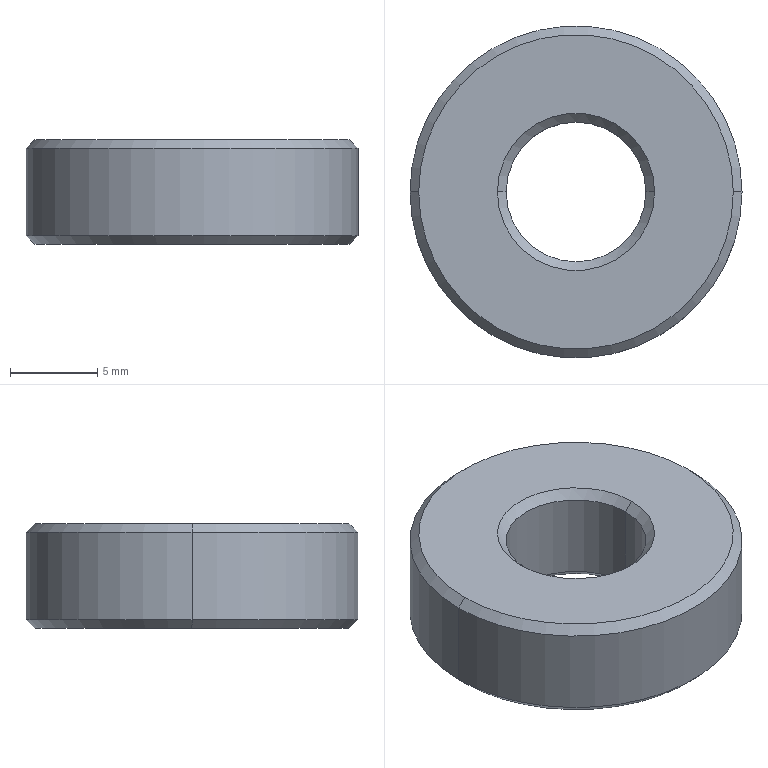Part | STEP file | QA-B698ZZ | 1 solid | 14 faces | box 19 x 19 x 6 mm | volume 1378 mm3 | cone 8 | cylinder 4 | plane 2 | commonest cylinder face diameters 8 x2 19 x2
STEP:
#1=CARTESIAN_POINT('',(0.,0.,0.));
#2=DIRECTION('',(0.,0.,1.));
#3=DIRECTION('',(1.,0.,0.));
#4=AXIS2_PLACEMENT_3D('',#1,#2,#3);
#5=CARTESIAN_POINT('',(4.,0.,5.5));
#6=VERTEX_POINT('',#5);
#7=CARTESIAN_POINT('',(4.5,0.,6.));
#8=VERTEX_POINT('',#7);
#9=CARTESIAN_POINT('',(4.,0.,5.5));
#10=DIRECTION('',(0.7071,0.,0.7071));
#11=VECTOR('',#10,1.);
#12=LINE('',#9,#11);
#13=CARTESIAN_POINT('',(0.,0.,5.5));
#14=DIRECTION('',(0.,0.,1.));
#15=DIRECTION('',(1.,0.,0.));
#16=AXIS2_PLACEMENT_3D('',#13,#14,#15);
#17=CONICAL_SURFACE('',#16,4.,0.7854);
#18=CARTESIAN_POINT('',(6.283,0.));
#19=DIRECTION('',(0.,1.));
#20=VECTOR('',#19,1.);
#21=LINE('',#18,#20);
#22=(GEOMETRIC_REPRESENTATION_CONTEXT(2)PARAMETRIC_REPRESENTATION_CONTEXT()REPRESENTATION_CONTEXT('',''));
#23=DEFINITIONAL_REPRESENTATION('',(#21),#22);
#24=PCURVE('',#17,#23);
#25=CARTESIAN_POINT('',(0.,0.,5.5));
#26=DIRECTION('',(0.,0.,1.));
#27=DIRECTION('',(1.,0.,0.));
#28=AXIS2_PLACEMENT_3D('',#25,#26,#27);
#29=CONICAL_SURFACE('',#28,4.,0.7854);
#30=CARTESIAN_POINT('',(0.,0.));
#31=DIRECTION('',(0.,1.));
#32=VECTOR('',#31,1.);
#33=LINE('',#30,#32);
#34=(GEOMETRIC_REPRESENTATION_CONTEXT(2)PARAMETRIC_REPRESENTATION_CONTEXT()REPRESENTATION_CONTEXT('',''));
#35=DEFINITIONAL_REPRESENTATION('',(#33),#34);
#36=PCURVE('',#29,#35);
#37=SURFACE_CURVE('',#12,(#24,#36),.PCURVE_S1.);
#38=EDGE_CURVE('',#6,#8,#37,.T.);
#39=ORIENTED_EDGE('',*,*,#38,.T.);
#40=CARTESIAN_POINT('',(-4.5,0.,6.));
#41=VERTEX_POINT('',#40);
#42=CARTESIAN_POINT('',(0.,0.,6.));
#43=DIRECTION('',(0.,0.,-1.));
#44=DIRECTION('',(1.,0.,0.));
#45=AXIS2_PLACEMENT_3D('',#42,#43,#44);
#46=CIRCLE('',#45,4.5);
#47=CARTESIAN_POINT('',(6.283,0.5));
#48=DIRECTION('',(-1.,0.));
#49=VECTOR('',#48,1.);
#50=LINE('',#47,#49);
#51=(GEOMETRIC_REPRESENTATION_CONTEXT(2)PARAMETRIC_REPRESENTATION_CONTEXT()REPRESENTATION_CONTEXT('',''));
#52=DEFINITIONAL_REPRESENTATION('',(#50),#51);
#53=PCURVE('',#17,#52);
#54=CARTESIAN_POINT('',(0.,0.,6.));
#55=DIRECTION('',(0.,0.,1.));
#56=DIRECTION('',(1.,0.,0.));
#57=AXIS2_PLACEMENT_3D('',#54,#55,#56);
#58=PLANE('',#57);
#59=CARTESIAN_POINT('',(4.5,0.));
#60=CARTESIAN_POINT('',(4.5,-7.794));
#61=CARTESIAN_POINT('',(-2.25,-3.897));
#62=CARTESIAN_POINT('',(-9.,0.));
#63=CARTESIAN_POINT('',(-2.25,3.897));
#64=CARTESIAN_POINT('',(4.5,7.794));
#65=CARTESIAN_POINT('',(4.5,0.));
#66=(BOUNDED_CURVE()B_SPLINE_CURVE(2,(#59,#60,#61,#62,#63,#64,#65),.UNSPECIFIED.,.T.,.F.)B_SPLINE_CURVE_WITH_KNOTS((1,2,2,2,2,1),(-2.094,0.,2.094,4.189,6.283,8.378),.UNSPECIFIED.)CURVE()GEOMETRIC_REPRESENTATION_ITEM()RATIONAL_B_SPLINE_CURVE((1.,0.5,1.,0.5,1.,0.5,1.))REPRESENTATION_ITEM(''));
#67=(GEOMETRIC_REPRESENTATION_CONTEXT(2)PARAMETRIC_REPRESENTATION_CONTEXT()REPRESENTATION_CONTEXT('',''));
#68=DEFINITIONAL_REPRESENTATION('',(#66),#67);
#69=PCURVE('',#58,#68);
#70=SURFACE_CURVE('',#46,(#53,#69),.PCURVE_S1.);
#71=EDGE_CURVE('',#8,#41,#70,.T.);
#72=ORIENTED_EDGE('',*,*,#71,.T.);
#73=CARTESIAN_POINT('',(-4.,0.,5.5));
#74=VERTEX_POINT('',#73);
#75=CARTESIAN_POINT('',(-4.,0.,5.5));
#76=DIRECTION('',(-0.7071,0.,0.7071));
#77=VECTOR('',#76,1.);
#78=LINE('',#75,#77);
#79=CARTESIAN_POINT('',(3.142,0.));
#80=DIRECTION('',(0.,1.));
#81=VECTOR('',#80,1.);
#82=LINE('',#79,#81);
#83=(GEOMETRIC_REPRESENTATION_CONTEXT(2)PARAMETRIC_REPRESENTATION_CONTEXT()REPRESENTATION_CONTEXT('',''));
#84=DEFINITIONAL_REPRESENTATION('',(#82),#83);
#85=PCURVE('',#17,#84);
#86=CARTESIAN_POINT('',(3.142,0.));
#87=DIRECTION('',(0.,1.));
#88=VECTOR('',#87,1.);
#89=LINE('',#86,#88);
#90=(GEOMETRIC_REPRESENTATION_CONTEXT(2)PARAMETRIC_REPRESENTATION_CONTEXT()REPRESENTATION_CONTEXT('',''));
#91=DEFINITIONAL_REPRESENTATION('',(#89),#90);
#92=PCURVE('',#29,#91);
#93=SURFACE_CURVE('',#78,(#85,#92),.PCURVE_S1.);
#94=EDGE_CURVE('',#74,#41,#93,.T.);
#95=ORIENTED_EDGE('',*,*,#94,.F.);
#96=CARTESIAN_POINT('',(0.,0.,5.5));
#97=DIRECTION('',(0.,0.,1.));
#98=DIRECTION('',(1.,0.,0.));
#99=AXIS2_PLACEMENT_3D('',#96,#97,#98);
#100=CIRCLE('',#99,4.);
#101=CARTESIAN_POINT('',(0.,0.));
#102=DIRECTION('',(1.,0.));
#103=VECTOR('',#102,1.);
#104=LINE('',#101,#103);
#105=(GEOMETRIC_REPRESENTATION_CONTEXT(2)PARAMETRIC_REPRESENTATION_CONTEXT()REPRESENTATION_CONTEXT('',''));
#106=DEFINITIONAL_REPRESENTATION('',(#104),#105);
#107=PCURVE('',#17,#106);
#108=CARTESIAN_POINT('',(0.,0.,6.));
#109=DIRECTION('',(0.,0.,-1.));
#110=DIRECTION('',(-1.,0.,0.));
#111=AXIS2_PLACEMENT_3D('',#108,#109,#110);
#112=CYLINDRICAL_SURFACE('',#111,4.);
#113=CARTESIAN_POINT('',(9.425,0.5));
#114=DIRECTION('',(-1.,0.));
#115=VECTOR('',#114,1.);
#116=LINE('',#113,#115);
#117=(GEOMETRIC_REPRESENTATION_CONTEXT(2)PARAMETRIC_REPRESENTATION_CONTEXT()REPRESENTATION_CONTEXT('',''));
#118=DEFINITIONAL_REPRESENTATION('',(#116),#117);
#119=PCURVE('',#112,#118);
#120=SURFACE_CURVE('',#100,(#107,#119),.PCURVE_S1.);
#121=EDGE_CURVE('',#74,#6,#120,.T.);
#122=ORIENTED_EDGE('',*,*,#121,.T.);
#123=EDGE_LOOP('',(#39,#72,#95,#122));
#124=FACE_BOUND('',#123,.F.);
#125=ADVANCED_FACE('',(#124),#17,.F.);
#126=CARTESIAN_POINT('',(-4.,0.,0.5));
#127=VERTEX_POINT('',#126);
#128=CARTESIAN_POINT('',(-4.5,0.,0.));
#129=VERTEX_POINT('',#128);
#130=CARTESIAN_POINT('',(-4.5,0.,0.));
#131=DIRECTION('',(-0.7071,0.,-0.7071));
#132=VECTOR('',#131,1.);
#133=LINE('',#130,#132);
#134=CARTESIAN_POINT('',(0.,0.,0.));
#135=DIRECTION('',(0.,0.,-1.));
#136=DIRECTION('',(-1.,0.,0.));
#137=AXIS2_PLACEMENT_3D('',#134,#135,#136);
#138=CONICAL_SURFACE('',#137,4.5,0.7854);
#139=CARTESIAN_POINT('',(6.283,0.));
#140=DIRECTION('',(0.,1.));
#141=VECTOR('',#140,1.);
#142=LINE('',#139,#141);
#143=(GEOMETRIC_REPRESENTATION_CONTEXT(2)PARAMETRIC_REPRESENTATION_CONTEXT()REPRESENTATION_CONTEXT('',''));
#144=DEFINITIONAL_REPRESENTATION('',(#142),#143);
#145=PCURVE('',#138,#144);
#146=CARTESIAN_POINT('',(0.,0.,0.));
#147=DIRECTION('',(0.,0.,-1.));
#148=DIRECTION('',(-1.,0.,0.));
#149=AXIS2_PLACEMENT_3D('',#146,#147,#148);
#150=CONICAL_SURFACE('',#149,4.5,0.7854);
#151=CARTESIAN_POINT('',(0.,0.));
#152=DIRECTION('',(0.,1.));
#153=VECTOR('',#152,1.);
#154=LINE('',#151,#153);
#155=(GEOMETRIC_REPRESENTATION_CONTEXT(2)PARAMETRIC_REPRESENTATION_CONTEXT()REPRESENTATION_CONTEXT('',''));
#156=DEFINITIONAL_REPRESENTATION('',(#154),#155);
#157=PCURVE('',#150,#156);
#158=SURFACE_CURVE('',#133,(#145,#157),.PCURVE_S1.);
#159=EDGE_CURVE('',#127,#129,#158,.T.);
#160=ORIENTED_EDGE('',*,*,#159,.T.);
#161=CARTESIAN_POINT('',(4.5,0.,0.));
#162=VERTEX_POINT('',#161);
#163=CARTESIAN_POINT('',(0.,0.,0.));
#164=DIRECTION('',(0.,0.,1.));
#165=DIRECTION('',(1.,0.,0.));
#166=AXIS2_PLACEMENT_3D('',#163,#164,#165);
#167=CIRCLE('',#166,4.5);
#168=CARTESIAN_POINT('',(9.425,0.));
#169=DIRECTION('',(-1.,0.));
#170=VECTOR('',#169,1.);
#171=LINE('',#168,#170);
#172=(GEOMETRIC_REPRESENTATION_CONTEXT(2)PARAMETRIC_REPRESENTATION_CONTEXT()REPRESENTATION_CONTEXT('',''));
#173=DEFINITIONAL_REPRESENTATION('',(#171),#172);
#174=PCURVE('',#138,#173);
#175=CARTESIAN_POINT('',(0.,0.,0.));
#176=DIRECTION('',(0.,0.,1.));
#177=DIRECTION('',(1.,0.,0.));
#178=AXIS2_PLACEMENT_3D('',#175,#176,#177);
#179=PLANE('',#178);
#180=CARTESIAN_POINT('',(0.,0.));
#181=DIRECTION('',(1.,0.));
#182=AXIS2_PLACEMENT_2D('',#180,#181);
#183=CIRCLE('',#182,4.5);
#184=(GEOMETRIC_REPRESENTATION_CONTEXT(2)PARAMETRIC_REPRESENTATION_CONTEXT()REPRESENTATION_CONTEXT('',''));
#185=DEFINITIONAL_REPRESENTATION('',(#183),#184);
#186=PCURVE('',#179,#185);
#187=SURFACE_CURVE('',#167,(#174,#186),.PCURVE_S1.);
#188=EDGE_CURVE('',#129,#162,#187,.T.);
#189=ORIENTED_EDGE('',*,*,#188,.T.);
#190=CARTESIAN_POINT('',(4.,0.,0.5));
#191=VERTEX_POINT('',#190);
#192=CARTESIAN_POINT('',(4.5,0.,0.));
#193=DIRECTION('',(0.7071,0.,-0.7071));
#194=VECTOR('',#193,1.);
#195=LINE('',#192,#194);
#196=CARTESIAN_POINT('',(3.142,0.));
#197=DIRECTION('',(0.,1.));
#198=VECTOR('',#197,1.);
#199=LINE('',#196,#198);
#200=(GEOMETRIC_REPRESENTATION_CONTEXT(2)PARAMETRIC_REPRESENTATION_CONTEXT()REPRESENTATION_CONTEXT('',''));
#201=DEFINITIONAL_REPRESENTATION('',(#199),#200);
#202=PCURVE('',#138,#201);
#203=CARTESIAN_POINT('',(3.142,0.));
#204=DIRECTION('',(0.,1.));
#205=VECTOR('',#204,1.);
#206=LINE('',#203,#205);
#207=(GEOMETRIC_REPRESENTATION_CONTEXT(2)PARAMETRIC_REPRESENTATION_CONTEXT()REPRESENTATION_CONTEXT('',''));
#208=DEFINITIONAL_REPRESENTATION('',(#206),#207);
#209=PCURVE('',#150,#208);
#210=SURFACE_CURVE('',#195,(#202,#209),.PCURVE_S1.);
#211=EDGE_CURVE('',#191,#162,#210,.T.);
#212=ORIENTED_EDGE('',*,*,#211,.F.);
#213=CARTESIAN_POINT('',(0.,0.,0.5));
#214=DIRECTION('',(0.,0.,-1.));
#215=DIRECTION('',(1.,0.,0.));
#216=AXIS2_PLACEMENT_3D('',#213,#214,#215);
#217=CIRCLE('',#216,4.);
#218=CARTESIAN_POINT('',(3.142,-0.5));
#219=DIRECTION('',(1.,0.));
#220=VECTOR('',#219,1.);
#221=LINE('',#218,#220);
#222=(GEOMETRIC_REPRESENTATION_CONTEXT(2)PARAMETRIC_REPRESENTATION_CONTEXT()REPRESENTATION_CONTEXT('',''));
#223=DEFINITIONAL_REPRESENTATION('',(#221),#222);
#224=PCURVE('',#138,#223);
#225=CARTESIAN_POINT('',(3.142,5.5));
#226=DIRECTION('',(1.,0.));
#227=VECTOR('',#226,1.);
#228=LINE('',#225,#227);
#229=(GEOMETRIC_REPRESENTATION_CONTEXT(2)PARAMETRIC_REPRESENTATION_CONTEXT()REPRESENTATION_CONTEXT('',''));
#230=DEFINITIONAL_REPRESENTATION('',(#228),#229);
#231=PCURVE('',#112,#230);
#232=SURFACE_CURVE('',#217,(#224,#231),.PCURVE_S1.);
#233=EDGE_CURVE('',#191,#127,#232,.T.);
#234=ORIENTED_EDGE('',*,*,#233,.T.);
#235=EDGE_LOOP('',(#160,#189,#212,#234));
#236=FACE_BOUND('',#235,.F.);
#237=ADVANCED_FACE('',(#236),#138,.F.);
#238=CARTESIAN_POINT('',(9.,0.,6.));
#239=VERTEX_POINT('',#238);
#240=CARTESIAN_POINT('',(-9.,0.,6.));
#241=VERTEX_POINT('',#240);
#242=CARTESIAN_POINT('',(0.,0.,6.));
#243=DIRECTION('',(0.,0.,1.));
#244=DIRECTION('',(1.,0.,0.));
#245=AXIS2_PLACEMENT_3D('',#242,#243,#244);
#246=CIRCLE('',#245,9.);
#247=CARTESIAN_POINT('',(0.,0.,6.));
#248=DIRECTION('',(0.,0.,-1.));
#249=DIRECTION('',(-1.,0.,0.));
#250=AXIS2_PLACEMENT_3D('',#247,#248,#249);
#251=CONICAL_SURFACE('',#250,9.,0.7854);
#252=CARTESIAN_POINT('',(3.142,0.));
#253=DIRECTION('',(-1.,0.));
#254=VECTOR('',#253,1.);
#255=LINE('',#252,#254);
#256=(GEOMETRIC_REPRESENTATION_CONTEXT(2)PARAMETRIC_REPRESENTATION_CONTEXT()REPRESENTATION_CONTEXT('',''));
#257=DEFINITIONAL_REPRESENTATION('',(#255),#256);
#258=PCURVE('',#251,#257);
#259=CARTESIAN_POINT('',(0.,0.));
#260=DIRECTION('',(1.,0.));
#261=AXIS2_PLACEMENT_2D('',#259,#260);
#262=CIRCLE('',#261,9.);
#263=(GEOMETRIC_REPRESENTATION_CONTEXT(2)PARAMETRIC_REPRESENTATION_CONTEXT()REPRESENTATION_CONTEXT('',''));
#264=DEFINITIONAL_REPRESENTATION('',(#262),#263);
#265=PCURVE('',#58,#264);
#266=SURFACE_CURVE('',#246,(#258,#265),.PCURVE_S1.);
#267=EDGE_CURVE('',#239,#241,#266,.T.);
#268=ORIENTED_EDGE('',*,*,#267,.F.);
#269=CARTESIAN_POINT('',(9.5,0.,5.5));
#270=VERTEX_POINT('',#269);
#271=CARTESIAN_POINT('',(9.,0.,6.));
#272=DIRECTION('',(0.7071,0.,-0.7071));
#273=VECTOR('',#272,1.);
#274=LINE('',#271,#273);
#275=CARTESIAN_POINT('',(3.142,0.));
#276=DIRECTION('',(0.,1.));
#277=VECTOR('',#276,1.);
#278=LINE('',#275,#277);
#279=(GEOMETRIC_REPRESENTATION_CONTEXT(2)PARAMETRIC_REPRESENTATION_CONTEXT()REPRESENTATION_CONTEXT('',''));
#280=DEFINITIONAL_REPRESENTATION('',(#278),#279);
#281=PCURVE('',#251,#280);
#282=CARTESIAN_POINT('',(0.,0.,6.));
#283=DIRECTION('',(0.,0.,-1.));
#284=DIRECTION('',(-1.,0.,0.));
#285=AXIS2_PLACEMENT_3D('',#282,#283,#284);
#286=CONICAL_SURFACE('',#285,9.,0.7854);
#287=CARTESIAN_POINT('',(3.142,0.));
#288=DIRECTION('',(0.,1.));
#289=VECTOR('',#288,1.);
#290=LINE('',#287,#289);
#291=(GEOMETRIC_REPRESENTATION_CONTEXT(2)PARAMETRIC_REPRESENTATION_CONTEXT()REPRESENTATION_CONTEXT('',''));
#292=DEFINITIONAL_REPRESENTATION('',(#290),#291);
#293=PCURVE('',#286,#292);
#294=SURFACE_CURVE('',#274,(#281,#293),.PCURVE_S1.);
#295=EDGE_CURVE('',#239,#270,#294,.T.);
#296=ORIENTED_EDGE('',*,*,#295,.T.);
#297=CARTESIAN_POINT('',(-9.5,0.,5.5));
#298=VERTEX_POINT('',#297);
#299=CARTESIAN_POINT('',(0.,0.,5.5));
#300=DIRECTION('',(0.,0.,-1.));
#301=DIRECTION('',(1.,0.,0.));
#302=AXIS2_PLACEMENT_3D('',#299,#300,#301);
#303=CIRCLE('',#302,9.5);
#304=CARTESIAN_POINT('',(-3.142,0.5));
#305=DIRECTION('',(1.,0.));
#306=VECTOR('',#305,1.);
#307=LINE('',#304,#306);
#308=(GEOMETRIC_REPRESENTATION_CONTEXT(2)PARAMETRIC_REPRESENTATION_CONTEXT()REPRESENTATION_CONTEXT('',''));
#309=DEFINITIONAL_REPRESENTATION('',(#307),#308);
#310=PCURVE('',#251,#309);
#311=CARTESIAN_POINT('',(0.,0.,6.));
#312=DIRECTION('',(0.,0.,-1.));
#313=DIRECTION('',(-1.,0.,0.));
#314=AXIS2_PLACEMENT_3D('',#311,#312,#313);
#315=CYLINDRICAL_SURFACE('',#314,9.5);
#316=CARTESIAN_POINT('',(-3.142,0.5));
#317=DIRECTION('',(1.,0.));
#318=VECTOR('',#317,1.);
#319=LINE('',#316,#318);
#320=(GEOMETRIC_REPRESENTATION_CONTEXT(2)PARAMETRIC_REPRESENTATION_CONTEXT()REPRESENTATION_CONTEXT('',''));
#321=DEFINITIONAL_REPRESENTATION('',(#319),#320);
#322=PCURVE('',#315,#321);
#323=SURFACE_CURVE('',#303,(#310,#322),.PCURVE_S1.);
#324=EDGE_CURVE('',#298,#270,#323,.T.);
#325=ORIENTED_EDGE('',*,*,#324,.F.);
#326=CARTESIAN_POINT('',(-9.,0.,6.));
#327=DIRECTION('',(-0.7071,0.,-0.7071));
#328=VECTOR('',#327,1.);
#329=LINE('',#326,#328);
#330=CARTESIAN_POINT('',(0.,0.));
#331=DIRECTION('',(0.,1.));
#332=VECTOR('',#331,1.);
#333=LINE('',#330,#332);
#334=(GEOMETRIC_REPRESENTATION_CONTEXT(2)PARAMETRIC_REPRESENTATION_CONTEXT()REPRESENTATION_CONTEXT('',''));
#335=DEFINITIONAL_REPRESENTATION('',(#333),#334);
#336=PCURVE('',#251,#335);
#337=CARTESIAN_POINT('',(6.283,0.));
#338=DIRECTION('',(0.,1.));
#339=VECTOR('',#338,1.);
#340=LINE('',#337,#339);
#341=(GEOMETRIC_REPRESENTATION_CONTEXT(2)PARAMETRIC_REPRESENTATION_CONTEXT()REPRESENTATION_CONTEXT('',''));
#342=DEFINITIONAL_REPRESENTATION('',(#340),#341);
#343=PCURVE('',#286,#342);
#344=SURFACE_CURVE('',#329,(#336,#343),.PCURVE_S1.);
#345=EDGE_CURVE('',#241,#298,#344,.T.);
#346=ORIENTED_EDGE('',*,*,#345,.F.);
#347=EDGE_LOOP('',(#268,#296,#325,#346));
#348=FACE_BOUND('',#347,.T.);
#349=ADVANCED_FACE('',(#348),#251,.T.);
#350=CARTESIAN_POINT('',(-9.,0.,0.));
#351=VERTEX_POINT('',#350);
#352=CARTESIAN_POINT('',(9.,0.,0.));
#353=VERTEX_POINT('',#352);
#354=CARTESIAN_POINT('',(0.,0.,0.));
#355=DIRECTION('',(0.,0.,-1.));
#356=DIRECTION('',(1.,0.,0.));
#357=AXIS2_PLACEMENT_3D('',#354,#355,#356);
#358=CIRCLE('',#357,9.);
#359=CARTESIAN_POINT('',(0.,0.,0.5));
#360=DIRECTION('',(0.,0.,1.));
#361=DIRECTION('',(1.,0.,0.));
#362=AXIS2_PLACEMENT_3D('',#359,#360,#361);
#363=CONICAL_SURFACE('',#362,9.5,0.7854);
#364=CARTESIAN_POINT('',(6.283,-0.5));
#365=DIRECTION('',(-1.,0.));
#366=VECTOR('',#365,1.);
#367=LINE('',#364,#366);
#368=(GEOMETRIC_REPRESENTATION_CONTEXT(2)PARAMETRIC_REPRESENTATION_CONTEXT()REPRESENTATION_CONTEXT('',''));
#369=DEFINITIONAL_REPRESENTATION('',(#367),#368);
#370=PCURVE('',#363,#369);
#371=CARTESIAN_POINT('',(9.,0.));
#372=CARTESIAN_POINT('',(9.,-15.588));
#373=CARTESIAN_POINT('',(-4.5,-7.794));
#374=CARTESIAN_POINT('',(-18.,0.));
#375=CARTESIAN_POINT('',(-4.5,7.794));
#376=CARTESIAN_POINT('',(9.,15.588));
#377=CARTESIAN_POINT('',(9.,0.));
#378=(BOUNDED_CURVE()B_SPLINE_CURVE(2,(#371,#372,#373,#374,#375,#376,#377),.UNSPECIFIED.,.T.,.F.)B_SPLINE_CURVE_WITH_KNOTS((1,2,2,2,2,1),(-2.094,0.,2.094,4.189,6.283,8.378),.UNSPECIFIED.)CURVE()GEOMETRIC_REPRESENTATION_ITEM()RATIONAL_B_SPLINE_CURVE((1.,0.5,1.,0.5,1.,0.5,1.))REPRESENTATION_ITEM(''));
#379=(GEOMETRIC_REPRESENTATION_CONTEXT(2)PARAMETRIC_REPRESENTATION_CONTEXT()REPRESENTATION_CONTEXT('',''));
#380=DEFINITIONAL_REPRESENTATION('',(#378),#379);
#381=PCURVE('',#179,#380);
#382=SURFACE_CURVE('',#358,(#370,#381),.PCURVE_S1.);
#383=EDGE_CURVE('',#351,#353,#382,.T.);
#384=ORIENTED_EDGE('',*,*,#383,.F.);
#385=CARTESIAN_POINT('',(-9.5,0.,0.5));
#386=VERTEX_POINT('',#385);
#387=CARTESIAN_POINT('',(-9.5,0.,0.5));
#388=DIRECTION('',(-0.7071,0.,0.7071));
#389=VECTOR('',#388,1.);
#390=LINE('',#387,#389);
#391=CARTESIAN_POINT('',(3.142,0.));
#392=DIRECTION('',(0.,1.));
#393=VECTOR('',#392,1.);
#394=LINE('',#391,#393);
#395=(GEOMETRIC_REPRESENTATION_CONTEXT(2)PARAMETRIC_REPRESENTATION_CONTEXT()REPRESENTATION_CONTEXT('',''));
#396=DEFINITIONAL_REPRESENTATION('',(#394),#395);
#397=PCURVE('',#363,#396);
#398=CARTESIAN_POINT('',(0.,0.,0.5));
#399=DIRECTION('',(0.,0.,1.));
#400=DIRECTION('',(1.,0.,0.));
#401=AXIS2_PLACEMENT_3D('',#398,#399,#400);
#402=CONICAL_SURFACE('',#401,9.5,0.7854);
#403=CARTESIAN_POINT('',(3.142,0.));
#404=DIRECTION('',(0.,1.));
#405=VECTOR('',#404,1.);
#406=LINE('',#403,#405);
#407=(GEOMETRIC_REPRESENTATION_CONTEXT(2)PARAMETRIC_REPRESENTATION_CONTEXT()REPRESENTATION_CONTEXT('',''));
#408=DEFINITIONAL_REPRESENTATION('',(#406),#407);
#409=PCURVE('',#402,#408);
#410=SURFACE_CURVE('',#390,(#397,#409),.PCURVE_S1.);
#411=EDGE_CURVE('',#351,#386,#410,.T.);
#412=ORIENTED_EDGE('',*,*,#411,.T.);
#413=CARTESIAN_POINT('',(9.5,0.,0.5));
#414=VERTEX_POINT('',#413);
#415=CARTESIAN_POINT('',(0.,0.,0.5));
#416=DIRECTION('',(0.,0.,1.));
#417=DIRECTION('',(1.,0.,0.));
#418=AXIS2_PLACEMENT_3D('',#415,#416,#417);
#419=CIRCLE('',#418,9.5);
#420=CARTESIAN_POINT('',(0.,0.));
#421=DIRECTION('',(1.,0.));
#422=VECTOR('',#421,1.);
#423=LINE('',#420,#422);
#424=(GEOMETRIC_REPRESENTATION_CONTEXT(2)PARAMETRIC_REPRESENTATION_CONTEXT()REPRESENTATION_CONTEXT('',''));
#425=DEFINITIONAL_REPRESENTATION('',(#423),#424);
#426=PCURVE('',#363,#425);
#427=CARTESIAN_POINT('',(3.142,5.5));
#428=DIRECTION('',(-1.,0.));
#429=VECTOR('',#428,1.);
#430=LINE('',#427,#429);
#431=(GEOMETRIC_REPRESENTATION_CONTEXT(2)PARAMETRIC_REPRESENTATION_CONTEXT()REPRESENTATION_CONTEXT('',''));
#432=DEFINITIONAL_REPRESENTATION('',(#430),#431);
#433=PCURVE('',#315,#432);
#434=SURFACE_CURVE('',#419,(#426,#433),.PCURVE_S1.);
#435=EDGE_CURVE('',#414,#386,#434,.T.);
#436=ORIENTED_EDGE('',*,*,#435,.F.);
#437=CARTESIAN_POINT('',(9.5,0.,0.5));
#438=DIRECTION('',(0.7071,0.,0.7071));
#439=VECTOR('',#438,1.);
#440=LINE('',#437,#439);
#441=CARTESIAN_POINT('',(0.,0.));
#442=DIRECTION('',(0.,1.));
#443=VECTOR('',#442,1.);
#444=LINE('',#441,#443);
#445=(GEOMETRIC_REPRESENTATION_CONTEXT(2)PARAMETRIC_REPRESENTATION_CONTEXT()REPRESENTATION_CONTEXT('',''));
#446=DEFINITIONAL_REPRESENTATION('',(#444),#445);
#447=PCURVE('',#363,#446);
#448=CARTESIAN_POINT('',(6.283,0.));
#449=DIRECTION('',(0.,1.));
#450=VECTOR('',#449,1.);
#451=LINE('',#448,#450);
#452=(GEOMETRIC_REPRESENTATION_CONTEXT(2)PARAMETRIC_REPRESENTATION_CONTEXT()REPRESENTATION_CONTEXT('',''));
#453=DEFINITIONAL_REPRESENTATION('',(#451),#452);
#454=PCURVE('',#402,#453);
#455=SURFACE_CURVE('',#440,(#447,#454),.PCURVE_S1.);
#456=EDGE_CURVE('',#353,#414,#455,.T.);
#457=ORIENTED_EDGE('',*,*,#456,.F.);
#458=EDGE_LOOP('',(#384,#412,#436,#457));
#459=FACE_BOUND('',#458,.T.);
#460=ADVANCED_FACE('',(#459),#363,.T.);
#461=CARTESIAN_POINT('',(-4.,0.,6.));
#462=DIRECTION('',(0.,0.,-1.));
#463=VECTOR('',#462,1.);
#464=LINE('',#461,#463);
#465=CARTESIAN_POINT('',(6.283,0.));
#466=DIRECTION('',(0.,1.));
#467=VECTOR('',#466,1.);
#468=LINE('',#465,#467);
#469=(GEOMETRIC_REPRESENTATION_CONTEXT(2)PARAMETRIC_REPRESENTATION_CONTEXT()REPRESENTATION_CONTEXT('',''));
#470=DEFINITIONAL_REPRESENTATION('',(#468),#469);
#471=PCURVE('',#112,#470);
#472=CARTESIAN_POINT('',(0.,0.,6.));
#473=DIRECTION('',(0.,0.,-1.));
#474=DIRECTION('',(-1.,0.,0.));
#475=AXIS2_PLACEMENT_3D('',#472,#473,#474);
#476=CYLINDRICAL_SURFACE('',#475,4.);
#477=CARTESIAN_POINT('',(0.,0.));
#478=DIRECTION('',(0.,1.));
#479=VECTOR('',#478,1.);
#480=LINE('',#477,#479);
#481=(GEOMETRIC_REPRESENTATION_CONTEXT(2)PARAMETRIC_REPRESENTATION_CONTEXT()REPRESENTATION_CONTEXT('',''));
#482=DEFINITIONAL_REPRESENTATION('',(#480),#481);
#483=PCURVE('',#476,#482);
#484=SURFACE_CURVE('',#464,(#471,#483),.PCURVE_S1.);
#485=EDGE_CURVE('',#74,#127,#484,.T.);
#486=ORIENTED_EDGE('',*,*,#485,.T.);
#487=ORIENTED_EDGE('',*,*,#233,.F.);
#488=CARTESIAN_POINT('',(4.,0.,6.));
#489=DIRECTION('',(0.,0.,-1.));
#490=VECTOR('',#489,1.);
#491=LINE('',#488,#490);
#492=CARTESIAN_POINT('',(3.142,0.));
#493=DIRECTION('',(0.,1.));
#494=VECTOR('',#493,1.);
#495=LINE('',#492,#494);
#496=(GEOMETRIC_REPRESENTATION_CONTEXT(2)PARAMETRIC_REPRESENTATION_CONTEXT()REPRESENTATION_CONTEXT('',''));
#497=DEFINITIONAL_REPRESENTATION('',(#495),#496);
#498=PCURVE('',#112,#497);
#499=CARTESIAN_POINT('',(3.142,0.));
#500=DIRECTION('',(0.,1.));
#501=VECTOR('',#500,1.);
#502=LINE('',#499,#501);
#503=(GEOMETRIC_REPRESENTATION_CONTEXT(2)PARAMETRIC_REPRESENTATION_CONTEXT()REPRESENTATION_CONTEXT('',''));
#504=DEFINITIONAL_REPRESENTATION('',(#502),#503);
#505=PCURVE('',#476,#504);
#506=SURFACE_CURVE('',#491,(#498,#505),.PCURVE_S1.);
#507=EDGE_CURVE('',#6,#191,#506,.T.);
#508=ORIENTED_EDGE('',*,*,#507,.F.);
#509=ORIENTED_EDGE('',*,*,#121,.F.);
#510=EDGE_LOOP('',(#486,#487,#508,#509));
#511=FACE_BOUND('',#510,.F.);
#512=ADVANCED_FACE('',(#511),#112,.F.);
#513=ORIENTED_EDGE('',*,*,#324,.T.);
#514=CARTESIAN_POINT('',(9.5,0.,6.));
#515=DIRECTION('',(0.,0.,-1.));
#516=VECTOR('',#515,1.);
#517=LINE('',#514,#516);
#518=CARTESIAN_POINT('',(3.142,0.));
#519=DIRECTION('',(0.,1.));
#520=VECTOR('',#519,1.);
#521=LINE('',#518,#520);
#522=(GEOMETRIC_REPRESENTATION_CONTEXT(2)PARAMETRIC_REPRESENTATION_CONTEXT()REPRESENTATION_CONTEXT('',''));
#523=DEFINITIONAL_REPRESENTATION('',(#521),#522);
#524=PCURVE('',#315,#523);
#525=CARTESIAN_POINT('',(0.,0.,6.));
#526=DIRECTION('',(0.,0.,-1.));
#527=DIRECTION('',(-1.,0.,0.));
#528=AXIS2_PLACEMENT_3D('',#525,#526,#527);
#529=CYLINDRICAL_SURFACE('',#528,9.5);
#530=CARTESIAN_POINT('',(3.142,0.));
#531=DIRECTION('',(0.,1.));
#532=VECTOR('',#531,1.);
#533=LINE('',#530,#532);
#534=(GEOMETRIC_REPRESENTATION_CONTEXT(2)PARAMETRIC_REPRESENTATION_CONTEXT()REPRESENTATION_CONTEXT('',''));
#535=DEFINITIONAL_REPRESENTATION('',(#533),#534);
#536=PCURVE('',#529,#535);
#537=SURFACE_CURVE('',#517,(#524,#536),.PCURVE_S1.);
#538=EDGE_CURVE('',#270,#414,#537,.T.);
#539=ORIENTED_EDGE('',*,*,#538,.T.);
#540=ORIENTED_EDGE('',*,*,#435,.T.);
#541=CARTESIAN_POINT('',(-9.5,0.,6.));
#542=DIRECTION('',(0.,0.,-1.));
#543=VECTOR('',#542,1.);
#544=LINE('',#541,#543);
#545=CARTESIAN_POINT('',(0.,0.));
#546=DIRECTION('',(0.,1.));
#547=VECTOR('',#546,1.);
#548=LINE('',#545,#547);
#549=(GEOMETRIC_REPRESENTATION_CONTEXT(2)PARAMETRIC_REPRESENTATION_CONTEXT()REPRESENTATION_CONTEXT('',''));
#550=DEFINITIONAL_REPRESENTATION('',(#548),#549);
#551=PCURVE('',#315,#550);
#552=CARTESIAN_POINT('',(6.283,0.));
#553=DIRECTION('',(0.,1.));
#554=VECTOR('',#553,1.);
#555=LINE('',#552,#554);
#556=(GEOMETRIC_REPRESENTATION_CONTEXT(2)PARAMETRIC_REPRESENTATION_CONTEXT()REPRESENTATION_CONTEXT('',''));
#557=DEFINITIONAL_REPRESENTATION('',(#555),#556);
#558=PCURVE('',#529,#557);
#559=SURFACE_CURVE('',#544,(#551,#558),.PCURVE_S1.);
#560=EDGE_CURVE('',#298,#386,#559,.T.);
#561=ORIENTED_EDGE('',*,*,#560,.F.);
#562=EDGE_LOOP('',(#513,#539,#540,#561));
#563=FACE_BOUND('',#562,.T.);
#564=ADVANCED_FACE('',(#563),#315,.T.);
#565=CARTESIAN_POINT('',(0.,0.,6.));
#566=DIRECTION('',(0.,0.,1.));
#567=DIRECTION('',(1.,0.,0.));
#568=AXIS2_PLACEMENT_3D('',#565,#566,#567);
#569=CIRCLE('',#568,9.);
#570=CARTESIAN_POINT('',(0.,0.));
#571=DIRECTION('',(1.,0.));
#572=AXIS2_PLACEMENT_2D('',#570,#571);
#573=CIRCLE('',#572,9.);
#574=(GEOMETRIC_REPRESENTATION_CONTEXT(2)PARAMETRIC_REPRESENTATION_CONTEXT()REPRESENTATION_CONTEXT('',''));
#575=DEFINITIONAL_REPRESENTATION('',(#573),#574);
#576=PCURVE('',#58,#575);
#577=CARTESIAN_POINT('',(9.425,0.));
#578=DIRECTION('',(-1.,0.));
#579=VECTOR('',#578,1.);
#580=LINE('',#577,#579);
#581=(GEOMETRIC_REPRESENTATION_CONTEXT(2)PARAMETRIC_REPRESENTATION_CONTEXT()REPRESENTATION_CONTEXT('',''));
#582=DEFINITIONAL_REPRESENTATION('',(#580),#581);
#583=PCURVE('',#286,#582);
#584=SURFACE_CURVE('',#569,(#576,#583),.PCURVE_S1.);
#585=EDGE_CURVE('',#241,#239,#584,.T.);
#586=ORIENTED_EDGE('',*,*,#585,.T.);
#587=ORIENTED_EDGE('',*,*,#267,.T.);
#588=EDGE_LOOP('',(#586,#587));
#589=FACE_BOUND('',#588,.T.);
#590=ORIENTED_EDGE('',*,*,#71,.T.);
#591=CARTESIAN_POINT('',(0.,0.,6.));
#592=DIRECTION('',(0.,0.,-1.));
#593=DIRECTION('',(1.,0.,0.));
#594=AXIS2_PLACEMENT_3D('',#591,#592,#593);
#595=CIRCLE('',#594,4.5);
#596=CARTESIAN_POINT('',(4.5,0.));
#597=CARTESIAN_POINT('',(4.5,-7.794));
#598=CARTESIAN_POINT('',(-2.25,-3.897));
#599=CARTESIAN_POINT('',(-9.,0.));
#600=CARTESIAN_POINT('',(-2.25,3.897));
#601=CARTESIAN_POINT('',(4.5,7.794));
#602=CARTESIAN_POINT('',(4.5,0.));
#603=(BOUNDED_CURVE()B_SPLINE_CURVE(2,(#596,#597,#598,#599,#600,#601,#602),.UNSPECIFIED.,.T.,.F.)B_SPLINE_CURVE_WITH_KNOTS((1,2,2,2,2,1),(-2.094,0.,2.094,4.189,6.283,8.378),.UNSPECIFIED.)CURVE()GEOMETRIC_REPRESENTATION_ITEM()RATIONAL_B_SPLINE_CURVE((1.,0.5,1.,0.5,1.,0.5,1.))REPRESENTATION_ITEM(''));
#604=(GEOMETRIC_REPRESENTATION_CONTEXT(2)PARAMETRIC_REPRESENTATION_CONTEXT()REPRESENTATION_CONTEXT('',''));
#605=DEFINITIONAL_REPRESENTATION('',(#603),#604);
#606=PCURVE('',#58,#605);
#607=CARTESIAN_POINT('',(6.283,0.5));
#608=DIRECTION('',(-1.,0.));
#609=VECTOR('',#608,1.);
#610=LINE('',#607,#609);
#611=(GEOMETRIC_REPRESENTATION_CONTEXT(2)PARAMETRIC_REPRESENTATION_CONTEXT()REPRESENTATION_CONTEXT('',''));
#612=DEFINITIONAL_REPRESENTATION('',(#610),#611);
#613=PCURVE('',#29,#612);
#614=SURFACE_CURVE('',#595,(#606,#613),.PCURVE_S1.);
#615=EDGE_CURVE('',#41,#8,#614,.T.);
#616=ORIENTED_EDGE('',*,*,#615,.T.);
#617=EDGE_LOOP('',(#590,#616));
#618=FACE_BOUND('',#617,.T.);
#619=ADVANCED_FACE('',(#589,#618),#58,.T.);
#620=CARTESIAN_POINT('',(0.,0.,0.));
#621=DIRECTION('',(0.,0.,-1.));
#622=DIRECTION('',(1.,0.,0.));
#623=AXIS2_PLACEMENT_3D('',#620,#621,#622);
#624=CIRCLE('',#623,9.);
#625=CARTESIAN_POINT('',(9.,0.));
#626=CARTESIAN_POINT('',(9.,-15.588));
#627=CARTESIAN_POINT('',(-4.5,-7.794));
#628=CARTESIAN_POINT('',(-18.,0.));
#629=CARTESIAN_POINT('',(-4.5,7.794));
#630=CARTESIAN_POINT('',(9.,15.588));
#631=CARTESIAN_POINT('',(9.,0.));
#632=(BOUNDED_CURVE()B_SPLINE_CURVE(2,(#625,#626,#627,#628,#629,#630,#631),.UNSPECIFIED.,.T.,.F.)B_SPLINE_CURVE_WITH_KNOTS((1,2,2,2,2,1),(-2.094,0.,2.094,4.189,6.283,8.378),.UNSPECIFIED.)CURVE()GEOMETRIC_REPRESENTATION_ITEM()RATIONAL_B_SPLINE_CURVE((1.,0.5,1.,0.5,1.,0.5,1.))REPRESENTATION_ITEM(''));
#633=(GEOMETRIC_REPRESENTATION_CONTEXT(2)PARAMETRIC_REPRESENTATION_CONTEXT()REPRESENTATION_CONTEXT('',''));
#634=DEFINITIONAL_REPRESENTATION('',(#632),#633);
#635=PCURVE('',#179,#634);
#636=CARTESIAN_POINT('',(6.283,-0.5));
#637=DIRECTION('',(-1.,0.));
#638=VECTOR('',#637,1.);
#639=LINE('',#636,#638);
#640=(GEOMETRIC_REPRESENTATION_CONTEXT(2)PARAMETRIC_REPRESENTATION_CONTEXT()REPRESENTATION_CONTEXT('',''));
#641=DEFINITIONAL_REPRESENTATION('',(#639),#640);
#642=PCURVE('',#402,#641);
#643=SURFACE_CURVE('',#624,(#635,#642),.PCURVE_S1.);
#644=EDGE_CURVE('',#353,#351,#643,.T.);
#645=ORIENTED_EDGE('',*,*,#644,.T.);
#646=ORIENTED_EDGE('',*,*,#383,.T.);
#647=EDGE_LOOP('',(#645,#646));
#648=FACE_BOUND('',#647,.T.);
#649=ORIENTED_EDGE('',*,*,#188,.T.);
#650=CARTESIAN_POINT('',(0.,0.,0.));
#651=DIRECTION('',(0.,0.,1.));
#652=DIRECTION('',(1.,0.,0.));
#653=AXIS2_PLACEMENT_3D('',#650,#651,#652);
#654=CIRCLE('',#653,4.5);
#655=CARTESIAN_POINT('',(0.,0.));
#656=DIRECTION('',(1.,0.));
#657=AXIS2_PLACEMENT_2D('',#655,#656);
#658=CIRCLE('',#657,4.5);
#659=(GEOMETRIC_REPRESENTATION_CONTEXT(2)PARAMETRIC_REPRESENTATION_CONTEXT()REPRESENTATION_CONTEXT('',''));
#660=DEFINITIONAL_REPRESENTATION('',(#658),#659);
#661=PCURVE('',#179,#660);
#662=CARTESIAN_POINT('',(3.142,0.));
#663=DIRECTION('',(-1.,0.));
#664=VECTOR('',#663,1.);
#665=LINE('',#662,#664);
#666=(GEOMETRIC_REPRESENTATION_CONTEXT(2)PARAMETRIC_REPRESENTATION_CONTEXT()REPRESENTATION_CONTEXT('',''));
#667=DEFINITIONAL_REPRESENTATION('',(#665),#666);
#668=PCURVE('',#150,#667);
#669=SURFACE_CURVE('',#654,(#661,#668),.PCURVE_S1.);
#670=EDGE_CURVE('',#162,#129,#669,.T.);
#671=ORIENTED_EDGE('',*,*,#670,.T.);
#672=EDGE_LOOP('',(#649,#671));
#673=FACE_BOUND('',#672,.T.);
#674=ADVANCED_FACE('',(#648,#673),#179,.F.);
#675=ORIENTED_EDGE('',*,*,#538,.F.);
#676=CARTESIAN_POINT('',(0.,0.,5.5));
#677=DIRECTION('',(0.,0.,-1.));
#678=DIRECTION('',(1.,0.,0.));
#679=AXIS2_PLACEMENT_3D('',#676,#677,#678);
#680=CIRCLE('',#679,9.5);
#681=CARTESIAN_POINT('',(3.142,0.5));
#682=DIRECTION('',(1.,0.));
#683=VECTOR('',#682,1.);
#684=LINE('',#681,#683);
#685=(GEOMETRIC_REPRESENTATION_CONTEXT(2)PARAMETRIC_REPRESENTATION_CONTEXT()REPRESENTATION_CONTEXT('',''));
#686=DEFINITIONAL_REPRESENTATION('',(#684),#685);
#687=PCURVE('',#529,#686);
#688=CARTESIAN_POINT('',(3.142,0.5));
#689=DIRECTION('',(1.,0.));
#690=VECTOR('',#689,1.);
#691=LINE('',#688,#690);
#692=(GEOMETRIC_REPRESENTATION_CONTEXT(2)PARAMETRIC_REPRESENTATION_CONTEXT()REPRESENTATION_CONTEXT('',''));
#693=DEFINITIONAL_REPRESENTATION('',(#691),#692);
#694=PCURVE('',#286,#693);
#695=SURFACE_CURVE('',#680,(#687,#694),.PCURVE_S1.);
#696=EDGE_CURVE('',#270,#298,#695,.T.);
#697=ORIENTED_EDGE('',*,*,#696,.T.);
#698=ORIENTED_EDGE('',*,*,#560,.T.);
#699=CARTESIAN_POINT('',(0.,0.,0.5));
#700=DIRECTION('',(0.,0.,1.));
#701=DIRECTION('',(1.,0.,0.));
#702=AXIS2_PLACEMENT_3D('',#699,#700,#701);
#703=CIRCLE('',#702,9.5);
#704=CARTESIAN_POINT('',(9.425,5.5));
#705=DIRECTION('',(-1.,0.));
#706=VECTOR('',#705,1.);
#707=LINE('',#704,#706);
#708=(GEOMETRIC_REPRESENTATION_CONTEXT(2)PARAMETRIC_REPRESENTATION_CONTEXT()REPRESENTATION_CONTEXT('',''));
#709=DEFINITIONAL_REPRESENTATION('',(#707),#708);
#710=PCURVE('',#529,#709);
#711=CARTESIAN_POINT('',(0.,0.));
#712=DIRECTION('',(1.,0.));
#713=VECTOR('',#712,1.);
#714=LINE('',#711,#713);
#715=(GEOMETRIC_REPRESENTATION_CONTEXT(2)PARAMETRIC_REPRESENTATION_CONTEXT()REPRESENTATION_CONTEXT('',''));
#716=DEFINITIONAL_REPRESENTATION('',(#714),#715);
#717=PCURVE('',#402,#716);
#718=SURFACE_CURVE('',#703,(#710,#717),.PCURVE_S1.);
#719=EDGE_CURVE('',#386,#414,#718,.T.);
#720=ORIENTED_EDGE('',*,*,#719,.T.);
#721=EDGE_LOOP('',(#675,#697,#698,#720));
#722=FACE_BOUND('',#721,.T.);
#723=ADVANCED_FACE('',(#722),#529,.T.);
#724=CARTESIAN_POINT('',(0.,0.,0.5));
#725=DIRECTION('',(0.,0.,-1.));
#726=DIRECTION('',(1.,0.,0.));
#727=AXIS2_PLACEMENT_3D('',#724,#725,#726);
#728=CIRCLE('',#727,4.);
#729=CARTESIAN_POINT('',(-3.142,5.5));
#730=DIRECTION('',(1.,0.));
#731=VECTOR('',#730,1.);
#732=LINE('',#729,#731);
#733=(GEOMETRIC_REPRESENTATION_CONTEXT(2)PARAMETRIC_REPRESENTATION_CONTEXT()REPRESENTATION_CONTEXT('',''));
#734=DEFINITIONAL_REPRESENTATION('',(#732),#733);
#735=PCURVE('',#476,#734);
#736=CARTESIAN_POINT('',(-3.142,-0.5));
#737=DIRECTION('',(1.,0.));
#738=VECTOR('',#737,1.);
#739=LINE('',#736,#738);
#740=(GEOMETRIC_REPRESENTATION_CONTEXT(2)PARAMETRIC_REPRESENTATION_CONTEXT()REPRESENTATION_CONTEXT('',''));
#741=DEFINITIONAL_REPRESENTATION('',(#739),#740);
#742=PCURVE('',#150,#741);
#743=SURFACE_CURVE('',#728,(#735,#742),.PCURVE_S1.);
#744=EDGE_CURVE('',#127,#191,#743,.T.);
#745=ORIENTED_EDGE('',*,*,#744,.F.);
#746=ORIENTED_EDGE('',*,*,#485,.F.);
#747=CARTESIAN_POINT('',(0.,0.,5.5));
#748=DIRECTION('',(0.,0.,1.));
#749=DIRECTION('',(1.,0.,0.));
#750=AXIS2_PLACEMENT_3D('',#747,#748,#749);
#751=CIRCLE('',#750,4.);
#752=CARTESIAN_POINT('',(3.142,0.5));
#753=DIRECTION('',(-1.,0.));
#754=VECTOR('',#753,1.);
#755=LINE('',#752,#754);
#756=(GEOMETRIC_REPRESENTATION_CONTEXT(2)PARAMETRIC_REPRESENTATION_CONTEXT()REPRESENTATION_CONTEXT('',''));
#757=DEFINITIONAL_REPRESENTATION('',(#755),#756);
#758=PCURVE('',#476,#757);
#759=CARTESIAN_POINT('',(0.,0.));
#760=DIRECTION('',(1.,0.));
#761=VECTOR('',#760,1.);
#762=LINE('',#759,#761);
#763=(GEOMETRIC_REPRESENTATION_CONTEXT(2)PARAMETRIC_REPRESENTATION_CONTEXT()REPRESENTATION_CONTEXT('',''));
#764=DEFINITIONAL_REPRESENTATION('',(#762),#763);
#765=PCURVE('',#29,#764);
#766=SURFACE_CURVE('',#751,(#758,#765),.PCURVE_S1.);
#767=EDGE_CURVE('',#6,#74,#766,.T.);
#768=ORIENTED_EDGE('',*,*,#767,.F.);
#769=ORIENTED_EDGE('',*,*,#507,.T.);
#770=EDGE_LOOP('',(#745,#746,#768,#769));
#771=FACE_BOUND('',#770,.F.);
#772=ADVANCED_FACE('',(#771),#476,.F.);
#773=ORIENTED_EDGE('',*,*,#411,.F.);
#774=ORIENTED_EDGE('',*,*,#644,.F.);
#775=ORIENTED_EDGE('',*,*,#456,.T.);
#776=ORIENTED_EDGE('',*,*,#719,.F.);
#777=EDGE_LOOP('',(#773,#774,#775,#776));
#778=FACE_BOUND('',#777,.T.);
#779=ADVANCED_FACE('',(#778),#402,.T.);
#780=ORIENTED_EDGE('',*,*,#295,.F.);
#781=ORIENTED_EDGE('',*,*,#585,.F.);
#782=ORIENTED_EDGE('',*,*,#345,.T.);
#783=ORIENTED_EDGE('',*,*,#696,.F.);
#784=EDGE_LOOP('',(#780,#781,#782,#783));
#785=FACE_BOUND('',#784,.T.);
#786=ADVANCED_FACE('',(#785),#286,.T.);
#787=ORIENTED_EDGE('',*,*,#670,.T.);
#788=ORIENTED_EDGE('',*,*,#159,.F.);
#789=ORIENTED_EDGE('',*,*,#744,.T.);
#790=ORIENTED_EDGE('',*,*,#211,.T.);
#791=EDGE_LOOP('',(#787,#788,#789,#790));
#792=FACE_BOUND('',#791,.F.);
#793=ADVANCED_FACE('',(#792),#150,.F.);
#794=ORIENTED_EDGE('',*,*,#615,.T.);
#795=ORIENTED_EDGE('',*,*,#38,.F.);
#796=ORIENTED_EDGE('',*,*,#767,.T.);
#797=ORIENTED_EDGE('',*,*,#94,.T.);
#798=EDGE_LOOP('',(#794,#795,#796,#797));
#799=FACE_BOUND('',#798,.F.);
#800=ADVANCED_FACE('',(#799),#29,.F.);
#801=CLOSED_SHELL('',(#125,#237,#349,#460,#512,#564,#619,#674,#723,#772,#779,#786,#793,#800));
#802=MANIFOLD_SOLID_BREP('',#801);
#803=(LENGTH_UNIT()NAMED_UNIT(*)SI_UNIT(.MILLI.,.METRE.));
#804=UNCERTAINTY_MEASURE_WITH_UNIT(LENGTH_MEASURE(0.0000001),#803,'','');
#805=(NAMED_UNIT(*)PLANE_ANGLE_UNIT()SI_UNIT($,.RADIAN.));
#806=(NAMED_UNIT(*)SI_UNIT($,.STERADIAN.)SOLID_ANGLE_UNIT());
#807=(GEOMETRIC_REPRESENTATION_CONTEXT(3)GLOBAL_UNCERTAINTY_ASSIGNED_CONTEXT((#804))GLOBAL_UNIT_ASSIGNED_CONTEXT((#803,#805,#806))REPRESENTATION_CONTEXT('',''));
#808=ADVANCED_BREP_SHAPE_REPRESENTATION('',(#4,#802),#807);